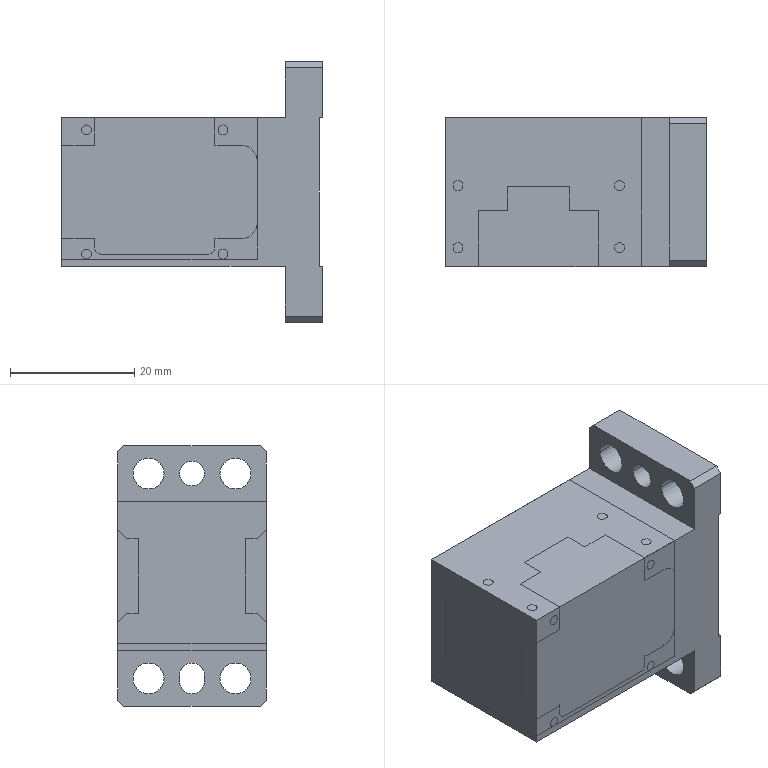NC program | NX | posted with a generic post | part box 42 x 24 x 42 mm
Lines 30711 to 31406 of 31406:
(DRILLING_1_COPY , TOOL : D3ZXZ)
N61402 T09 M6
N61404 G54
N61406 G17 G0 G90 X10. Y5. B0. C0. S5000 M3
N61408 G43 Z30. H9
N61410 G94 G81 G98 Z-1.1 F250. R3.
N61412 X7.5 Y1.5 Z-10.1 R-6.
N61414 Y-13.5
N61416 X10. Y-17. Z-1.1 R3.
N61418 X-10.
N61420 X-7.5 Y-13.5 Z-10.1 R-6.
N61422 Y1.5
N61424 X-10. Y5. Z-1.1 R3.
N61426 G80
N61428 G0 X-10. Y5. Z30.
N61430 M5
(DRILLING_COPY_COPY , TOOL : 1.6ZT)
N61432 T16 M6
N61434 G54
N61436 G17 G0 G90 X10. Y-17. B0. C0. S2000 M3
N61438 G43 Z30. H16
N61440 G94 G83 G98 Z-5.681 F100. Q2. R3.
N61442 X7.5 Y-13.5 Z-14.681 R-6.
N61444 Y1.5
N61446 X10. Y5. Z-5.681 R3.
N61448 X-10.
N61450 X-7.5 Y1.5 Z-14.681 R-6.
N61452 Y-13.5
N61454 X-10. Y-17. Z-5.681 R3.
N61456 G80
N61458 G0 X-10. Y-17. Z30.
N61460 M5
(ZLEVEL_PROFILE_2 , TOOL : D4R0.5)
N61462 T05 M6
N61464 G54
N61466 G17 G0 G90 X5.003 Y2.581 B0. C0. S7500 M3
N61468 G43 Z30. H5
N61470 Z0.929
N61472 G94 G1 Z-0.071 F3000.
N61474 X5.523 Y2.882
N61476 G3 X5.723 Y3.228 R0.4
N61478 G1 X5.72 Y7.1
N61480 X5.709 Y7.963
N61482 G3 X4.958 Y8.71 R0.756
N61484 G1 X3.227 Y8.721
N61486 X-3.789 Y8.72
N61488 X-4.958 Y8.711
N61490 G3 X-5.707 Y7.959 R0.755
N61492 G1 X-5.723 Y3.228
N61494 X-5.687 Z-0.106
N61496 X-5.652 Z-0.141
N61498 X-5.649 Y7.659
N61500 X-5.645 Y7.977
N61502 G2 X-4.963 Y8.65 R0.682
N61504 G1 X3.227 Y8.651
N61506 X4.975 Y8.648
N61508 G2 X5.647 Y7.982 R0.674
N61510 G1 X5.651 Y7.659
N61512 X5.652 Y3.228
N61514 X5.616 Z-0.177
N61516 X5.581 Z-0.212
N61518 Y3.7
N61520 Y8.
N61522 G3 X5. Y8.581 R0.581
N61524 G1 X-5.
N61526 G3 X-5.581 Y8. R0.581
N61528 G1 Y3.7
N61530 Y3.228
N61532 X-5.545 Z-0.247
N61534 X-5.51 Z-0.283
N61536 Y3.7
N61538 Y8.
N61540 G2 X-5. Y8.51 R0.51
N61542 G1 X5.
N61544 G2 X5.51 Y8. R0.51
N61546 G1 Y3.7
N61548 Y3.228
N61550 X5.475 Z-0.318
N61552 X5.44 Z-0.354
N61554 X5.439 Y3.7
N61556 Y8.
N61558 G3 X5. Y8.439 R0.439
N61560 G1 X-5.
N61562 G3 X-5.439 Y8. R0.439
N61564 G1 Y3.7
N61566 X-5.44 Y3.228
N61568 X-5.404 Z-0.389
N61570 X-5.369 Z-0.424
N61572 Y3.7
N61574 Y8.
N61576 G2 X-5. Y8.369 R0.369
N61578 G1 X5.
N61580 G2 X5.369 Y8. R0.369
N61582 G1 Y3.7
N61584 Y3.228
N61586 X5.333 Z-0.46
N61588 X5.298 Z-0.495
N61590 Y3.7
N61592 Y8.
N61594 G3 X5. Y8.298 R0.298
N61596 G1 X-5.
N61598 G3 X-5.298 Y8. R0.298
N61600 G1 Y3.7
N61602 Y3.228
N61604 X-5.263 Z-0.53
N61606 X-5.228 Z-0.566
N61608 X-5.227 Y3.7
N61610 Y8.
N61612 G2 X-5. Y8.227 R0.227
N61614 G1 X5.
N61616 G2 X5.227 Y8. R0.227
N61618 G1 Y3.7
N61620 X5.228 Y3.228
N61622 X5.192 Z-0.601
N61624 X5.157 Z-0.636
N61626 X5.156 Y3.7
N61628 Y8.
N61630 G3 X5. Y8.156 R0.156
N61632 G1 X-5.
N61634 G3 X-5.156 Y8. R0.156
N61636 G1 Y3.7
N61638 X-5.157 Y3.228
N61640 X-5.121 Z-0.672
N61642 X-5.086 Z-0.707
N61644 Y3.7
N61646 Y8.
N61648 X-5.083 Y8.048
N61650 X-5.048 Y8.083
N61652 X-5. Y8.086
N61654 X5.
N61656 X5.048 Y8.083
N61658 X5.083 Y8.048
N61660 X5.086 Y8.
N61662 Y3.7
N61664 Y3.228
N61666 X5.05 Z-0.742
N61668 X5.015 Z-0.778
N61670 Y3.7
N61672 Y8.
N61674 X5.016 Y8.016
N61676 X5. Y8.015
N61678 X-5.
N61680 X-5.016 Y8.016
N61682 X-5.015 Y8.
N61684 Y3.7
N61686 Y3.228
N61688 X-4.98 Z-0.813
N61690 X-4.945 Y3.227 Z-0.849
N61692 X-4.944 Y3.7
N61694 Y7.944
N61696 X4.944
N61698 Y3.7
N61700 X4.945 Y3.227
N61702 X4.909 Z-0.884
N61704 X4.874 Z-0.919
N61706 Y3.7
N61708 Y7.874
N61710 X-4.874
N61712 Y3.7
N61714 Y3.227
N61716 X-4.838 Z-0.955
N61718 X-4.803 Z-0.99
N61720 Y3.7
N61722 Y7.803
N61724 X4.803
N61726 Y3.7
N61728 Y3.227
N61730 X4.768 Y3.228 Z-1.025
N61732 X4.733 Z-1.061
N61734 X4.732 Y3.7
N61736 Y7.732
N61738 X-4.732
N61740 Y3.7
N61742 X-4.733 Y3.228
N61744 X-4.697 Z-1.096
N61746 X-4.662 Z-1.131
N61748 Y3.7
N61750 Y7.662
N61752 X4.662
N61754 Y3.7
N61756 Y3.228
N61758 X4.626 Z-1.167
N61760 X4.591 Z-1.202
N61762 Y3.7
N61764 Y7.591
N61766 X-4.591
N61768 Y3.7
N61770 Y3.228
N61772 X-4.555 Z-1.237
N61774 X-4.52 Z-1.273
N61776 Y3.7
N61778 Y7.52
N61780 X4.52
N61782 Y3.7
N61784 Y3.228
N61786 X4.485 Z-1.308
N61788 X4.45 Z-1.344
N61790 X4.449 Y3.7
N61792 Y7.449
N61794 X-4.449
N61796 Y3.7
N61798 X-4.45 Y3.228
N61800 X-4.414 Z-1.379
N61802 X-4.379 Z-1.414
N61804 Y3.7
N61806 Y7.379
N61808 X4.379
N61810 Y3.7
N61812 Y3.228
N61814 X4.343 Z-1.45
N61816 X4.308 Z-1.485
N61818 Y3.7
N61820 Y7.308
N61822 X-4.308
N61824 Y3.7
N61826 Y3.228
N61828 X-4.273 Z-1.52
N61830 X-4.238 Z-1.556
N61832 X-4.237 Y3.7
N61834 Y7.237
N61836 X4.237
N61838 Y3.7
N61840 X4.238 Y3.228
N61842 X4.202 Z-1.591
N61844 X4.167 Z-1.626
N61846 Y3.7
N61848 Y7.167
N61850 X-4.167
N61852 Y3.7
N61854 Y3.228
N61856 X-4.131 Z-1.662
N61858 X-4.096 Z-1.697
N61860 Y6.821
N61862 X-4.093 Y7.092
N61864 X-3.508 Y7.094
N61866 X4.069 Y7.096
N61868 X4.092 Y7.093
N61870 X4.095 Y6.541
N61872 X4.096 Y3.228
N61874 X4.026 Y3.269 Z-1.768
N61876 X4.024 Y6.541
N61878 X4.021 Y7.021
N61880 X3.789 Y7.024
N61882 X-3.227 Y7.025
N61884 X-4.021 Y7.02
N61886 X-4.024 Y6.821
N61888 X-4.026 Y3.269
N61890 X-3.968 Y3.323 Z-1.826
N61892 X-3.965 Y6.821
N61894 X-3.962 Y6.962
N61896 X-3.508 Y6.965
N61898 X3.789 Y6.964
N61900 X3.963 Y6.962
N61902 X3.966 Y6.541
N61904 X3.968 Y3.323
N61906 X3.909 Y3.377 Z-1.884
N61908 X3.908 Y6.541
N61910 X3.905 Y6.903
N61912 X3.227 Y6.908
N61914 X-3.508 Y6.907
N61916 X-3.903 Y6.904
N61918 X-3.906 Y6.821
N61920 X-3.909 Y3.377
N61922 X-3.851 Y3.431 Z-1.942
N61924 X-3.847 Y6.821
N61926 X-3.845 Y6.846
N61928 X-3.508 Y6.849
N61930 X3.508 Y6.848
N61932 X3.848 Y6.843
N61934 X3.85 Y6.541
N61936 X3.851 Y3.431
N61938 G2 X3.651 Y3.085 R0.4
N61940 G1 X3.093 Y2.762
N61942 Z-0.942
N61944 G0 Z30.
N61946 X2.993 Y5.464
N61948 Z-1.
N61950 G1 Z-2.
N61952 X3.594 Y5.816
N61954 G3 X3.792 Y6.163 R0.4
N61956 G1 X3.789 Y6.787
N61958 X3.227 Y6.791
N61960 X-3.508
N61962 X-3.789 Y6.789
N61964 X-3.791 Y6.214
N61966 G3 X-3.593 Y5.867 R0.4
N61968 G1 X-2.992 Y5.517
N61970 Z-1.
N61972 G0 Z30.
N61974 X-5.002 Y-14.581
N61976 Z0.929
N61978 G1 Z-0.071
N61980 X-5.523 Y-14.882
N61982 G3 X-5.723 Y-15.228 R0.4
N61984 G1 Y-21.472
N61986 X-5.687 Z-0.106
N61988 X-5.652 Z-0.141
N61990 X-5.653 Y-15.228
N61992 X-5.616 Z-0.177
N61994 X-5.582 Z-0.212
N61996 X-5.581 Y-15.7
N61998 Y-21.
N62000 Y-21.472
N62002 X-5.545 Z-0.247
N62004 X-5.511 Z-0.283
N62006 X-5.51 Y-21.
N62008 Y-15.7
N62010 X-5.511 Y-15.228
N62012 X-5.475 Z-0.318
N62014 X-5.44 Z-0.354
N62016 X-5.439 Y-15.7
N62018 Y-21.
N62020 X-5.44 Y-21.472
N62022 X-5.404 Z-0.389
N62024 X-5.369 Z-0.424
N62026 Y-21.
N62028 Y-15.7
N62030 X-5.37 Y-15.228
N62032 X-5.333 Z-0.46
N62034 X-5.299 Z-0.495
N62036 X-5.298 Y-15.7
N62038 Y-21.
N62040 Y-21.472
N62042 X-5.263 Z-0.53
N62044 X-5.228 Z-0.566
N62046 X-5.227 Y-21.
N62048 Y-15.7
N62050 X-5.228 Y-15.228
N62052 X-5.192 Z-0.601
N62054 X-5.158 Z-0.636
N62056 X-5.156 Y-15.7
N62058 Y-21.
N62060 X-5.157 Y-21.472
N62062 X-5.121 Z-0.672
N62064 X-5.086 Z-0.707
N62066 Y-21.
N62068 Y-15.7
N62070 X-5.087 Y-15.228
N62072 X-5.05 Z-0.742
N62074 X-5.016 Z-0.778
N62076 X-5.015 Y-15.7
N62078 Y-21.
N62080 X-5.016 Y-21.472
N62082 X-4.98 Z-0.813
N62084 X-4.945 Y-21.473 Z-0.849
N62086 X-4.944 Y-21.
N62088 Y-15.7
N62090 X-4.945 Y-15.227
N62092 X-4.909 Z-0.884
N62094 X-4.875 Z-0.919
N62096 X-4.874 Y-15.7
N62098 Y-21.
N62100 Y-21.472
N62102 X-4.838 Z-0.955
N62104 X-4.803 Z-0.99
N62106 Y-21.
N62108 Y-15.7
N62110 X-4.804 Y-15.228
N62112 X-4.768 Z-1.025
N62114 X-4.733 Z-1.061
N62116 X-4.732 Y-15.7
N62118 Y-21.
N62120 X-4.733 Y-21.472
N62122 X-4.697 Z-1.096
N62124 X-4.662 Z-1.131
N62126 Y-21.
N62128 Y-15.7
N62130 X-4.663 Y-15.228
N62132 X-4.626 Z-1.167
N62134 X-4.592 Z-1.202
N62136 X-4.591 Y-15.7
N62138 Y-21.
N62140 Y-21.472
N62142 X-4.555 Z-1.237
N62144 X-4.521 Z-1.273
N62146 X-4.52 Y-21.
N62148 Y-15.7
N62150 X-4.521 Y-15.228
N62152 X-4.485 Z-1.308
N62154 X-4.45 Z-1.344
N62156 X-4.449 Y-15.7
N62158 Y-21.
N62160 X-4.45 Y-21.472
N62162 X-4.414 Z-1.379
N62164 X-4.379 Z-1.414
N62166 Y-21.
N62168 Y-15.7
N62170 X-4.38 Y-15.228
N62172 X-4.343 Z-1.45
N62174 X-4.309 Z-1.485
N62176 X-4.308 Y-15.7
N62178 Y-21.
N62180 X-4.309 Y-21.472
N62182 X-4.273 Z-1.52
N62184 X-4.238 Z-1.556
N62186 X-4.237 Y-21.
N62188 Y-15.7
N62190 X-4.238 Y-15.228
N62192 X-4.202 Z-1.591
N62194 X-4.168 Z-1.626
N62196 X-4.167 Y-15.7
N62198 Y-21.
N62200 Y-21.472
N62202 X-4.131 Z-1.662
N62204 X-4.096 Z-1.697
N62206 X-4.097 Y-15.228
N62208 X-4.026 Y-15.277 Z-1.768
N62210 Y-21.417
N62212 X-3.967 Y-21.37 Z-1.826
N62214 X-3.968 Y-15.32
N62216 X-3.909 Y-15.362 Z-1.884
N62218 Y-21.322
N62220 X-3.851 Y-21.275 Z-1.942
N62222 Y-15.405
N62224 G2 X-3.651 Y-15.058 R0.4
N62226 G1 X-3.096 Y-14.738
N62228 Z-0.942
N62230 G0 Z30.
N62232 X5.002 Y-22.118
N62234 Z0.929
N62236 G1 Z-0.071
N62238 X5.523 Y-21.818
N62240 G3 X5.723 Y-21.472 R0.4
N62242 G1 Y-15.228
N62244 X5.687 Z-0.106
N62246 X5.653 Z-0.141
N62248 X5.652 Y-21.472
N62250 X5.616 Z-0.177
N62252 X5.581 Z-0.212
N62254 Y-21.
N62256 Y-15.7
N62258 X5.582 Y-15.228
N62260 X5.545 Z-0.247
N62262 X5.511 Z-0.283
N62264 X5.51 Y-15.7
N62266 Y-21.
N62268 X5.511 Y-21.472
N62270 X5.475 Z-0.318
N62272 X5.44 Z-0.354
N62274 X5.439 Y-21.
N62276 Y-15.7
N62278 X5.44 Y-15.228
N62280 X5.404 Z-0.389
N62282 X5.37 Z-0.424
N62284 X5.369 Y-15.7
N62286 Y-21.
N62288 Y-21.472
N62290 X5.333 Z-0.46
N62292 X5.298 Z-0.495
N62294 Y-21.
N62296 Y-15.7
N62298 X5.299 Y-15.228
N62300 X5.263 Z-0.53
N62302 X5.228 Z-0.566
N62304 X5.227 Y-15.7
N62306 Y-21.
N62308 X5.228 Y-21.472
N62310 X5.192 Z-0.601
N62312 X5.157 Z-0.636
N62314 X5.156 Y-21.
N62316 Y-15.7
N62318 X5.158 Y-15.228
N62320 X5.121 Z-0.672
N62322 X5.087 Z-0.707
N62324 X5.086 Y-15.7
N62326 Y-21.
N62328 Y-21.472
N62330 X5.05 Z-0.742
N62332 X5.016 Z-0.778
N62334 X5.015 Y-21.
N62336 Y-15.7
N62338 X5.016 Y-15.228
N62340 X4.98 Y-15.227 Z-0.813
N62342 X4.945 Z-0.849
N62344 X4.944 Y-15.7
N62346 Y-21.
N62348 X4.945 Y-21.473
N62350 X4.909 Y-21.472 Z-0.884
N62352 X4.874 Z-0.919
N62354 Y-21.
N62356 Y-15.7
N62358 X4.875 Y-15.227
N62360 X4.838 Y-15.228 Z-0.955
N62362 X4.804 Z-0.99
N62364 X4.803 Y-15.7
N62366 Y-21.
N62368 Y-21.472
N62370 X4.768 Z-1.025
N62372 X4.733 Z-1.061
N62374 X4.732 Y-21.
N62376 Y-15.7
N62378 X4.733 Y-15.228
N62380 X4.697 Z-1.096
N62382 X4.663 Z-1.131
N62384 X4.662 Y-15.7
N62386 Y-21.
N62388 Y-21.472
N62390 X4.626 Z-1.167
N62392 X4.591 Z-1.202
N62394 Y-21.
N62396 Y-15.7
N62398 X4.592 Y-15.228
N62400 X4.555 Z-1.237
N62402 X4.521 Z-1.273
N62404 X4.52 Y-15.7
N62406 Y-21.
N62408 X4.521 Y-21.472
N62410 X4.485 Z-1.308
N62412 X4.45 Z-1.344
N62414 X4.449 Y-21.
N62416 Y-15.7
N62418 X4.45 Y-15.228
N62420 X4.414 Z-1.379
N62422 X4.38 Z-1.414
N62424 X4.379 Y-15.7
N62426 Y-21.
N62428 Y-21.472
N62430 X4.343 Z-1.45
N62432 X4.309 Z-1.485
N62434 X4.308 Y-21.
N62436 Y-15.7
N62438 X4.309 Y-15.228
N62440 X4.273 Z-1.52
N62442 X4.238 Z-1.556
N62444 X4.237 Y-15.7
N62446 Y-21.
N62448 X4.238 Y-21.472
N62450 X4.202 Z-1.591
N62452 X4.167 Z-1.626
N62454 Y-21.
N62456 Y-15.7
N62458 X4.168 Y-15.228
N62460 X4.131 Z-1.662
N62462 X4.097 Z-1.697
N62464 X4.096 Y-21.472
N62466 X4.026 Y-21.417 Z-1.768
N62468 Y-15.277
N62470 X3.968 Y-15.32 Z-1.826
N62472 X3.967 Y-21.37
N62474 X3.909 Y-21.322 Z-1.884
N62476 Y-15.362
N62478 X3.851 Y-15.405 Z-1.942
N62480 Y-21.275
N62482 G2 X3.651 Y-21.622 R0.4
N62484 G1 X3.093 Y-21.944
N62486 Z-0.942
N62488 G0 Z30.
N62490 M5
(PLANAR_MILL_COPY_2_COPY_1 , TOOL : D6A45)
N62492 T07 M6
N62494 G54
N62496 G17 G0 G90 X-13.27 Y-13.6 B0. C0. S7500 M3
N62498 G43 Z30. H7
N62500 Z0.5
N62502 G94 G1 Z-1. F1250.
N62504 X-12.866 Y-14.3
N62506 G3 X-12. Y-14.8 R1.
N62508 G1 X-7.5
N62510 G3 X-6.634 Y-14.3 R1.
N62512 G1 X-6.23 Y-13.6
N62514 Z0.5
N62516 G0 Z30.
N62518 X6.23
N62520 Z0.5
N62522 G1 Z-1.
N62524 X6.634 Y-14.3
N62526 G3 X7.5 Y-14.8 R1.
N62528 G1 X9.
N62530 X9.065 Y-14.813
N62532 X9.113 Y-14.765
N62534 X9.1 Y-14.7
N62536 Y2.7
N62538 X9.113 Y2.765
N62540 X9.065 Y2.813
N62542 X9. Y2.8
N62544 X7.5
N62546 G3 X6.634 Y2.3 R1.
N62548 G1 X6.23 Y1.6
N62550 Z0.5
N62552 G0 Z30.
N62554 X-6.23
N62556 Z0.5
N62558 G1 Z-1.
N62560 X-6.634 Y2.3
N62562 G3 X-7.5 Y2.8 R1.
N62564 G1 X-12.
N62566 G3 X-12.866 Y2.3 R1.
N62568 G1 X-13.27 Y1.6
N62570 Z0.5
N62572 G0 Z30.
N62574 M5
(刀补6 , TOOL : D6JING)
N62576 T15 M6
N62578 G54
N62580 G17 G0 G90 X1.696 Y-14.706 B0. C0. S7500 M3
N62582 G43 Z30. H15
N62584 Z-7.
N62586 G94 G1 Z-8. F1000.
N62588 G41 X1.73 Y-14.8 D15
N62590 X2.134 Y-15.5
N62592 G3 X3. Y-16. R1.
N62594 G1 Y4.
N62596 X-3.
N62598 Y-16.
N62600 X3.
N62602 G3 X2.5 Y-15.134 R1.
N62604 G1 X1.8 Y-14.73
N62606 G40
N62608 X1.706 Y-14.696
N62610 Z-7.
N62612 G0 Z3.
N62614 X1.696 Y-14.706
N62616 Z-15.
N62618 G1 Z-16.
N62620 G41 X1.73 Y-14.8
N62622 X2.134 Y-15.5
N62624 G3 X3. Y-16. R1.
N62626 G1 Y4.
N62628 X-3.
N62630 Y-16.
N62632 X3.
N62634 G3 X2.5 Y-15.134 R1.
N62636 G1 X1.8 Y-14.73
N62638 G40
N62640 X1.706 Y-14.696
N62642 Z-15.
N62644 G0 Z-5.
N62646 X1.696 Y-14.706
N62648 Z-23.
N62650 G1 Z-24.
N62652 G41 X1.73 Y-14.8
N62654 X2.134 Y-15.5
N62656 G3 X3. Y-16. R1.
N62658 G1 Y4.
N62660 X-3.
N62662 Y-16.
N62664 X3.
N62666 G3 X2.5 Y-15.134 R1.
N62668 G1 X1.8 Y-14.73
N62670 G40
N62672 X1.706 Y-14.696
N62674 Z-23.
N62676 G0 Z30.
(刀补66 , TOOL : D6JING)
N62678 X1.877 Y-22.219
N62680 Z-2.43
N62682 G1 Z-3.43
N62684 G41 X1.971 Y-22.185
N62686 X2.502 Y-21.876
N62688 G3 X3. Y-21.008 R1.
N62690 G1 Y-15.7
N62692 G2 X3.021 Y-15.344 R3.
N62694 G1 X3.02 Y-10.994
N62696 Y-10.877
N62698 X3.023 Y-10.833
N62700 Y-1.205
N62702 X3.021 Y-0.989
N62704 X3.02 Y3.352
N62706 G2 X3.002 Y3.581 R3.
N62708 G1 X3. Y3.7
N62710 Y6.
N62712 X-3.
N62714 Y3.7
N62716 X-3.003 Y3.572
N62718 G2 X-3.022 Y3.337 R3.
N62720 G1 X-3.023 Y2.594
N62722 Y-0.86
N62724 X-3.02 Y-1.001
N62726 X-3.023 Y-1.205
N62728 Y-10.531
N62730 X-3.022 Y-10.877
N62732 X-3.021 Y-11.006
N62734 X-3.023 Y-11.222
N62736 Y-15.328
N62738 G2 X-3. Y-15.7 R3.
N62740 G1 Y-21.008
N62742 G3 X-2.502 Y-21.876 R1.
N62744 G1 X-1.971 Y-22.185
N62746 G40
N62748 X-1.877 Y-22.219
N62750 Z-2.43
N62752 G0 Z30.
N62754 M5
N62756 M2